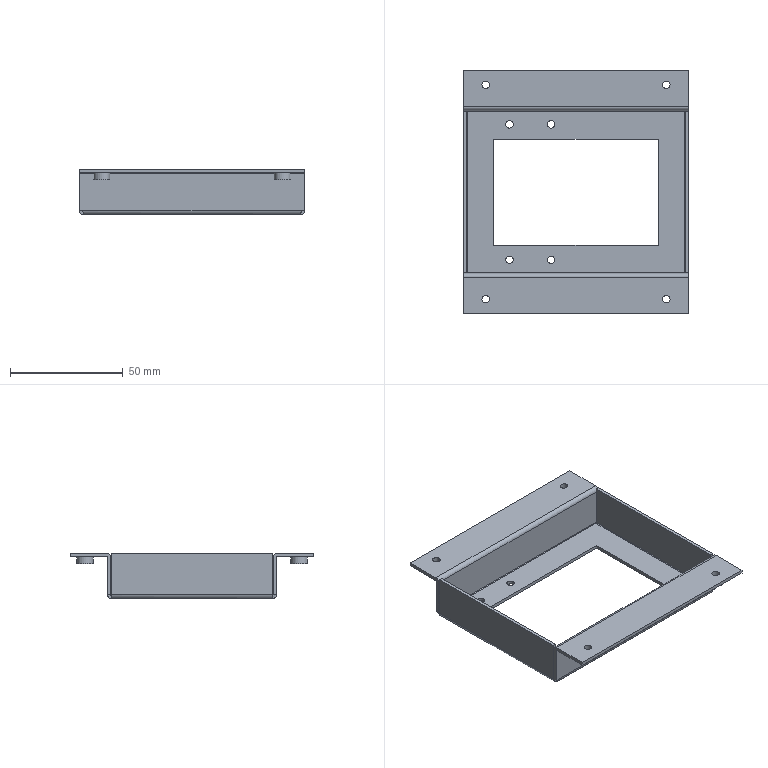Part | STEP file | FHD-021-008-01-A circuit breaker bracket 1 | 1 solid | 74 faces | box 100 x 108 x 20 mm | volume 20485 mm3 | plane 42 | cylinder 24 | spline 8 | commonest cylinder face diameters 3.3 x8 0.6 x6 3.6 x6 7.3 x4